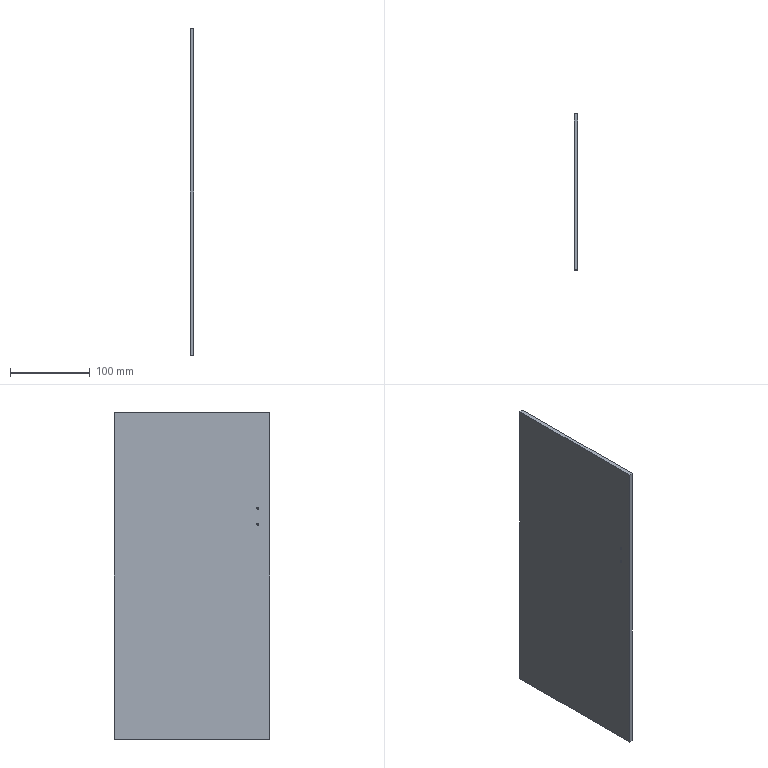Part | STEP file | 09-08 Outer side plate 1 | 1 solid | 10 faces | box 5 x 195 x 410 mm | volume 399701 mm3 | plane 6 | cylinder 4 | commonest cylinder face diameters 2.5 x4
STEP:
#1=CARTESIAN_POINT('',(0.,0.,0.));
#2=DIRECTION('',(0.,0.,1.));
#3=DIRECTION('',(1.,0.,0.));
#4=AXIS2_PLACEMENT_3D('',#1,#2,#3);
#5=CARTESIAN_POINT('',(0.,15.,-121.25));
#6=VERTEX_POINT('',#5);
#7=CARTESIAN_POINT('',(5.,15.,-121.25));
#8=VERTEX_POINT('',#7);
#9=CARTESIAN_POINT('',(0.,15.,-121.25));
#10=DIRECTION('',(1.,0.,0.));
#11=VECTOR('',#10,1.);
#12=LINE('',#9,#11);
#13=CARTESIAN_POINT('',(0.,15.,-120.));
#14=DIRECTION('',(1.,0.,0.));
#15=DIRECTION('',(0.,0.,-1.));
#16=AXIS2_PLACEMENT_3D('',#13,#14,#15);
#17=CYLINDRICAL_SURFACE('',#16,1.25);
#18=CARTESIAN_POINT('',(6.283,0.));
#19=DIRECTION('',(0.,1.));
#20=VECTOR('',#19,1.);
#21=LINE('',#18,#20);
#22=(GEOMETRIC_REPRESENTATION_CONTEXT(2)PARAMETRIC_REPRESENTATION_CONTEXT()REPRESENTATION_CONTEXT('',''));
#23=DEFINITIONAL_REPRESENTATION('',(#21),#22);
#24=PCURVE('',#17,#23);
#25=CARTESIAN_POINT('',(0.,15.,-120.));
#26=DIRECTION('',(1.,0.,0.));
#27=DIRECTION('',(0.,0.,-1.));
#28=AXIS2_PLACEMENT_3D('',#25,#26,#27);
#29=CYLINDRICAL_SURFACE('',#28,1.25);
#30=CARTESIAN_POINT('',(0.,0.));
#31=DIRECTION('',(0.,1.));
#32=VECTOR('',#31,1.);
#33=LINE('',#30,#32);
#34=(GEOMETRIC_REPRESENTATION_CONTEXT(2)PARAMETRIC_REPRESENTATION_CONTEXT()REPRESENTATION_CONTEXT('',''));
#35=DEFINITIONAL_REPRESENTATION('',(#33),#34);
#36=PCURVE('',#29,#35);
#37=SURFACE_CURVE('',#12,(#24,#36),.PCURVE_S1.);
#38=EDGE_CURVE('',#6,#8,#37,.T.);
#39=ORIENTED_EDGE('',*,*,#38,.T.);
#40=CARTESIAN_POINT('',(5.,15.,-118.75));
#41=VERTEX_POINT('',#40);
#42=CARTESIAN_POINT('',(5.,15.,-120.));
#43=DIRECTION('',(1.,0.,0.));
#44=DIRECTION('',(0.,0.,-1.));
#45=AXIS2_PLACEMENT_3D('',#42,#43,#44);
#46=CIRCLE('',#45,1.25);
#47=CARTESIAN_POINT('',(0.,5.));
#48=DIRECTION('',(1.,0.));
#49=VECTOR('',#48,1.);
#50=LINE('',#47,#49);
#51=(GEOMETRIC_REPRESENTATION_CONTEXT(2)PARAMETRIC_REPRESENTATION_CONTEXT()REPRESENTATION_CONTEXT('',''));
#52=DEFINITIONAL_REPRESENTATION('',(#50),#51);
#53=PCURVE('',#17,#52);
#54=CARTESIAN_POINT('',(5.,0.,-410.));
#55=DIRECTION('',(-1.,0.,0.));
#56=DIRECTION('',(0.,0.,1.));
#57=AXIS2_PLACEMENT_3D('',#54,#55,#56);
#58=PLANE('',#57);
#59=CARTESIAN_POINT('',(288.75,15.));
#60=CARTESIAN_POINT('',(288.75,17.165));
#61=CARTESIAN_POINT('',(290.625,16.083));
#62=CARTESIAN_POINT('',(292.5,15.));
#63=CARTESIAN_POINT('',(290.625,13.917));
#64=CARTESIAN_POINT('',(288.75,12.835));
#65=CARTESIAN_POINT('',(288.75,15.));
#66=(BOUNDED_CURVE()B_SPLINE_CURVE(2,(#59,#60,#61,#62,#63,#64,#65),.UNSPECIFIED.,.T.,.F.)B_SPLINE_CURVE_WITH_KNOTS((1,2,2,2,2,1),(-2.094,0.,2.094,4.189,6.283,8.378),.UNSPECIFIED.)CURVE()GEOMETRIC_REPRESENTATION_ITEM()RATIONAL_B_SPLINE_CURVE((1.,0.5,1.,0.5,1.,0.5,1.))REPRESENTATION_ITEM(''));
#67=(GEOMETRIC_REPRESENTATION_CONTEXT(2)PARAMETRIC_REPRESENTATION_CONTEXT()REPRESENTATION_CONTEXT('',''));
#68=DEFINITIONAL_REPRESENTATION('',(#66),#67);
#69=PCURVE('',#58,#68);
#70=SURFACE_CURVE('',#46,(#53,#69),.PCURVE_S1.);
#71=EDGE_CURVE('',#41,#8,#70,.T.);
#72=ORIENTED_EDGE('',*,*,#71,.F.);
#73=CARTESIAN_POINT('',(0.,15.,-118.75));
#74=VERTEX_POINT('',#73);
#75=CARTESIAN_POINT('',(0.,15.,-118.75));
#76=DIRECTION('',(1.,0.,0.));
#77=VECTOR('',#76,1.);
#78=LINE('',#75,#77);
#79=CARTESIAN_POINT('',(3.142,0.));
#80=DIRECTION('',(0.,1.));
#81=VECTOR('',#80,1.);
#82=LINE('',#79,#81);
#83=(GEOMETRIC_REPRESENTATION_CONTEXT(2)PARAMETRIC_REPRESENTATION_CONTEXT()REPRESENTATION_CONTEXT('',''));
#84=DEFINITIONAL_REPRESENTATION('',(#82),#83);
#85=PCURVE('',#17,#84);
#86=CARTESIAN_POINT('',(3.142,0.));
#87=DIRECTION('',(0.,1.));
#88=VECTOR('',#87,1.);
#89=LINE('',#86,#88);
#90=(GEOMETRIC_REPRESENTATION_CONTEXT(2)PARAMETRIC_REPRESENTATION_CONTEXT()REPRESENTATION_CONTEXT('',''));
#91=DEFINITIONAL_REPRESENTATION('',(#89),#90);
#92=PCURVE('',#29,#91);
#93=SURFACE_CURVE('',#78,(#85,#92),.PCURVE_S1.);
#94=EDGE_CURVE('',#74,#41,#93,.T.);
#95=ORIENTED_EDGE('',*,*,#94,.F.);
#96=CARTESIAN_POINT('',(0.,15.,-120.));
#97=DIRECTION('',(-1.,0.,0.));
#98=DIRECTION('',(0.,0.,-1.));
#99=AXIS2_PLACEMENT_3D('',#96,#97,#98);
#100=CIRCLE('',#99,1.25);
#101=CARTESIAN_POINT('',(6.283,0.));
#102=DIRECTION('',(-1.,0.));
#103=VECTOR('',#102,1.);
#104=LINE('',#101,#103);
#105=(GEOMETRIC_REPRESENTATION_CONTEXT(2)PARAMETRIC_REPRESENTATION_CONTEXT()REPRESENTATION_CONTEXT('',''));
#106=DEFINITIONAL_REPRESENTATION('',(#104),#105);
#107=PCURVE('',#17,#106);
#108=CARTESIAN_POINT('',(0.,0.,-410.));
#109=DIRECTION('',(-1.,0.,0.));
#110=DIRECTION('',(0.,0.,1.));
#111=AXIS2_PLACEMENT_3D('',#108,#109,#110);
#112=PLANE('',#111);
#113=CARTESIAN_POINT('',(290.,15.));
#114=DIRECTION('',(-1.,0.));
#115=AXIS2_PLACEMENT_2D('',#113,#114);
#116=CIRCLE('',#115,1.25);
#117=(GEOMETRIC_REPRESENTATION_CONTEXT(2)PARAMETRIC_REPRESENTATION_CONTEXT()REPRESENTATION_CONTEXT('',''));
#118=DEFINITIONAL_REPRESENTATION('',(#116),#117);
#119=PCURVE('',#112,#118);
#120=SURFACE_CURVE('',#100,(#107,#119),.PCURVE_S1.);
#121=EDGE_CURVE('',#6,#74,#120,.T.);
#122=ORIENTED_EDGE('',*,*,#121,.F.);
#123=EDGE_LOOP('',(#39,#72,#95,#122));
#124=FACE_BOUND('',#123,.F.);
#125=ADVANCED_FACE('',(#124),#17,.F.);
#126=CARTESIAN_POINT('',(0.,15.,-141.25));
#127=VERTEX_POINT('',#126);
#128=CARTESIAN_POINT('',(5.,15.,-141.25));
#129=VERTEX_POINT('',#128);
#130=CARTESIAN_POINT('',(0.,15.,-141.25));
#131=DIRECTION('',(1.,0.,0.));
#132=VECTOR('',#131,1.);
#133=LINE('',#130,#132);
#134=CARTESIAN_POINT('',(0.,15.,-140.));
#135=DIRECTION('',(1.,0.,0.));
#136=DIRECTION('',(0.,0.,-1.));
#137=AXIS2_PLACEMENT_3D('',#134,#135,#136);
#138=CYLINDRICAL_SURFACE('',#137,1.25);
#139=CARTESIAN_POINT('',(6.283,0.));
#140=DIRECTION('',(0.,1.));
#141=VECTOR('',#140,1.);
#142=LINE('',#139,#141);
#143=(GEOMETRIC_REPRESENTATION_CONTEXT(2)PARAMETRIC_REPRESENTATION_CONTEXT()REPRESENTATION_CONTEXT('',''));
#144=DEFINITIONAL_REPRESENTATION('',(#142),#143);
#145=PCURVE('',#138,#144);
#146=CARTESIAN_POINT('',(0.,15.,-140.));
#147=DIRECTION('',(1.,0.,0.));
#148=DIRECTION('',(0.,0.,-1.));
#149=AXIS2_PLACEMENT_3D('',#146,#147,#148);
#150=CYLINDRICAL_SURFACE('',#149,1.25);
#151=CARTESIAN_POINT('',(0.,0.));
#152=DIRECTION('',(0.,1.));
#153=VECTOR('',#152,1.);
#154=LINE('',#151,#153);
#155=(GEOMETRIC_REPRESENTATION_CONTEXT(2)PARAMETRIC_REPRESENTATION_CONTEXT()REPRESENTATION_CONTEXT('',''));
#156=DEFINITIONAL_REPRESENTATION('',(#154),#155);
#157=PCURVE('',#150,#156);
#158=SURFACE_CURVE('',#133,(#145,#157),.PCURVE_S1.);
#159=EDGE_CURVE('',#127,#129,#158,.T.);
#160=ORIENTED_EDGE('',*,*,#159,.T.);
#161=CARTESIAN_POINT('',(5.,15.,-138.75));
#162=VERTEX_POINT('',#161);
#163=CARTESIAN_POINT('',(5.,15.,-140.));
#164=DIRECTION('',(1.,0.,0.));
#165=DIRECTION('',(0.,0.,-1.));
#166=AXIS2_PLACEMENT_3D('',#163,#164,#165);
#167=CIRCLE('',#166,1.25);
#168=CARTESIAN_POINT('',(0.,5.));
#169=DIRECTION('',(1.,0.));
#170=VECTOR('',#169,1.);
#171=LINE('',#168,#170);
#172=(GEOMETRIC_REPRESENTATION_CONTEXT(2)PARAMETRIC_REPRESENTATION_CONTEXT()REPRESENTATION_CONTEXT('',''));
#173=DEFINITIONAL_REPRESENTATION('',(#171),#172);
#174=PCURVE('',#138,#173);
#175=CARTESIAN_POINT('',(268.75,15.));
#176=CARTESIAN_POINT('',(268.75,17.165));
#177=CARTESIAN_POINT('',(270.625,16.083));
#178=CARTESIAN_POINT('',(272.5,15.));
#179=CARTESIAN_POINT('',(270.625,13.917));
#180=CARTESIAN_POINT('',(268.75,12.835));
#181=CARTESIAN_POINT('',(268.75,15.));
#182=(BOUNDED_CURVE()B_SPLINE_CURVE(2,(#175,#176,#177,#178,#179,#180,#181),.UNSPECIFIED.,.T.,.F.)B_SPLINE_CURVE_WITH_KNOTS((1,2,2,2,2,1),(-2.094,0.,2.094,4.189,6.283,8.378),.UNSPECIFIED.)CURVE()GEOMETRIC_REPRESENTATION_ITEM()RATIONAL_B_SPLINE_CURVE((1.,0.5,1.,0.5,1.,0.5,1.))REPRESENTATION_ITEM(''));
#183=(GEOMETRIC_REPRESENTATION_CONTEXT(2)PARAMETRIC_REPRESENTATION_CONTEXT()REPRESENTATION_CONTEXT('',''));
#184=DEFINITIONAL_REPRESENTATION('',(#182),#183);
#185=PCURVE('',#58,#184);
#186=SURFACE_CURVE('',#167,(#174,#185),.PCURVE_S1.);
#187=EDGE_CURVE('',#162,#129,#186,.T.);
#188=ORIENTED_EDGE('',*,*,#187,.F.);
#189=CARTESIAN_POINT('',(0.,15.,-138.75));
#190=VERTEX_POINT('',#189);
#191=CARTESIAN_POINT('',(0.,15.,-138.75));
#192=DIRECTION('',(1.,0.,0.));
#193=VECTOR('',#192,1.);
#194=LINE('',#191,#193);
#195=CARTESIAN_POINT('',(3.142,0.));
#196=DIRECTION('',(0.,1.));
#197=VECTOR('',#196,1.);
#198=LINE('',#195,#197);
#199=(GEOMETRIC_REPRESENTATION_CONTEXT(2)PARAMETRIC_REPRESENTATION_CONTEXT()REPRESENTATION_CONTEXT('',''));
#200=DEFINITIONAL_REPRESENTATION('',(#198),#199);
#201=PCURVE('',#138,#200);
#202=CARTESIAN_POINT('',(3.142,0.));
#203=DIRECTION('',(0.,1.));
#204=VECTOR('',#203,1.);
#205=LINE('',#202,#204);
#206=(GEOMETRIC_REPRESENTATION_CONTEXT(2)PARAMETRIC_REPRESENTATION_CONTEXT()REPRESENTATION_CONTEXT('',''));
#207=DEFINITIONAL_REPRESENTATION('',(#205),#206);
#208=PCURVE('',#150,#207);
#209=SURFACE_CURVE('',#194,(#201,#208),.PCURVE_S1.);
#210=EDGE_CURVE('',#190,#162,#209,.T.);
#211=ORIENTED_EDGE('',*,*,#210,.F.);
#212=CARTESIAN_POINT('',(0.,15.,-140.));
#213=DIRECTION('',(1.,0.,0.));
#214=DIRECTION('',(0.,0.,-1.));
#215=AXIS2_PLACEMENT_3D('',#212,#213,#214);
#216=CIRCLE('',#215,1.25);
#217=CARTESIAN_POINT('',(0.,0.));
#218=DIRECTION('',(1.,0.));
#219=VECTOR('',#218,1.);
#220=LINE('',#217,#219);
#221=(GEOMETRIC_REPRESENTATION_CONTEXT(2)PARAMETRIC_REPRESENTATION_CONTEXT()REPRESENTATION_CONTEXT('',''));
#222=DEFINITIONAL_REPRESENTATION('',(#220),#221);
#223=PCURVE('',#138,#222);
#224=CARTESIAN_POINT('',(268.75,15.));
#225=CARTESIAN_POINT('',(268.75,17.165));
#226=CARTESIAN_POINT('',(270.625,16.083));
#227=CARTESIAN_POINT('',(272.5,15.));
#228=CARTESIAN_POINT('',(270.625,13.917));
#229=CARTESIAN_POINT('',(268.75,12.835));
#230=CARTESIAN_POINT('',(268.75,15.));
#231=(BOUNDED_CURVE()B_SPLINE_CURVE(2,(#224,#225,#226,#227,#228,#229,#230),.UNSPECIFIED.,.T.,.F.)B_SPLINE_CURVE_WITH_KNOTS((1,2,2,2,2,1),(-2.094,0.,2.094,4.189,6.283,8.378),.UNSPECIFIED.)CURVE()GEOMETRIC_REPRESENTATION_ITEM()RATIONAL_B_SPLINE_CURVE((1.,0.5,1.,0.5,1.,0.5,1.))REPRESENTATION_ITEM(''));
#232=(GEOMETRIC_REPRESENTATION_CONTEXT(2)PARAMETRIC_REPRESENTATION_CONTEXT()REPRESENTATION_CONTEXT('',''));
#233=DEFINITIONAL_REPRESENTATION('',(#231),#232);
#234=PCURVE('',#112,#233);
#235=SURFACE_CURVE('',#216,(#223,#234),.PCURVE_S1.);
#236=EDGE_CURVE('',#190,#127,#235,.T.);
#237=ORIENTED_EDGE('',*,*,#236,.T.);
#238=EDGE_LOOP('',(#160,#188,#211,#237));
#239=FACE_BOUND('',#238,.F.);
#240=ADVANCED_FACE('',(#239),#138,.F.);
#241=CARTESIAN_POINT('',(5.,15.,-120.));
#242=DIRECTION('',(1.,0.,0.));
#243=DIRECTION('',(0.,0.,-1.));
#244=AXIS2_PLACEMENT_3D('',#241,#242,#243);
#245=CIRCLE('',#244,1.25);
#246=CARTESIAN_POINT('',(0.,5.));
#247=DIRECTION('',(1.,0.));
#248=VECTOR('',#247,1.);
#249=LINE('',#246,#248);
#250=(GEOMETRIC_REPRESENTATION_CONTEXT(2)PARAMETRIC_REPRESENTATION_CONTEXT()REPRESENTATION_CONTEXT('',''));
#251=DEFINITIONAL_REPRESENTATION('',(#249),#250);
#252=PCURVE('',#29,#251);
#253=CARTESIAN_POINT('',(288.75,15.));
#254=CARTESIAN_POINT('',(288.75,17.165));
#255=CARTESIAN_POINT('',(290.625,16.083));
#256=CARTESIAN_POINT('',(292.5,15.));
#257=CARTESIAN_POINT('',(290.625,13.917));
#258=CARTESIAN_POINT('',(288.75,12.835));
#259=CARTESIAN_POINT('',(288.75,15.));
#260=(BOUNDED_CURVE()B_SPLINE_CURVE(2,(#253,#254,#255,#256,#257,#258,#259),.UNSPECIFIED.,.T.,.F.)B_SPLINE_CURVE_WITH_KNOTS((1,2,2,2,2,1),(-2.094,0.,2.094,4.189,6.283,8.378),.UNSPECIFIED.)CURVE()GEOMETRIC_REPRESENTATION_ITEM()RATIONAL_B_SPLINE_CURVE((1.,0.5,1.,0.5,1.,0.5,1.))REPRESENTATION_ITEM(''));
#261=(GEOMETRIC_REPRESENTATION_CONTEXT(2)PARAMETRIC_REPRESENTATION_CONTEXT()REPRESENTATION_CONTEXT('',''));
#262=DEFINITIONAL_REPRESENTATION('',(#260),#261);
#263=PCURVE('',#58,#262);
#264=SURFACE_CURVE('',#245,(#252,#263),.PCURVE_S1.);
#265=EDGE_CURVE('',#8,#41,#264,.T.);
#266=ORIENTED_EDGE('',*,*,#265,.F.);
#267=ORIENTED_EDGE('',*,*,#38,.F.);
#268=CARTESIAN_POINT('',(0.,15.,-120.));
#269=DIRECTION('',(-1.,0.,0.));
#270=DIRECTION('',(0.,0.,-1.));
#271=AXIS2_PLACEMENT_3D('',#268,#269,#270);
#272=CIRCLE('',#271,1.25);
#273=CARTESIAN_POINT('',(6.283,0.));
#274=DIRECTION('',(-1.,0.));
#275=VECTOR('',#274,1.);
#276=LINE('',#273,#275);
#277=(GEOMETRIC_REPRESENTATION_CONTEXT(2)PARAMETRIC_REPRESENTATION_CONTEXT()REPRESENTATION_CONTEXT('',''));
#278=DEFINITIONAL_REPRESENTATION('',(#276),#277);
#279=PCURVE('',#29,#278);
#280=CARTESIAN_POINT('',(290.,15.));
#281=DIRECTION('',(-1.,0.));
#282=AXIS2_PLACEMENT_2D('',#280,#281);
#283=CIRCLE('',#282,1.25);
#284=(GEOMETRIC_REPRESENTATION_CONTEXT(2)PARAMETRIC_REPRESENTATION_CONTEXT()REPRESENTATION_CONTEXT('',''));
#285=DEFINITIONAL_REPRESENTATION('',(#283),#284);
#286=PCURVE('',#112,#285);
#287=SURFACE_CURVE('',#272,(#279,#286),.PCURVE_S1.);
#288=EDGE_CURVE('',#74,#6,#287,.T.);
#289=ORIENTED_EDGE('',*,*,#288,.F.);
#290=ORIENTED_EDGE('',*,*,#94,.T.);
#291=EDGE_LOOP('',(#266,#267,#289,#290));
#292=FACE_BOUND('',#291,.F.);
#293=ADVANCED_FACE('',(#292),#29,.F.);
#294=CARTESIAN_POINT('',(5.,15.,-140.));
#295=DIRECTION('',(1.,0.,0.));
#296=DIRECTION('',(0.,0.,-1.));
#297=AXIS2_PLACEMENT_3D('',#294,#295,#296);
#298=CIRCLE('',#297,1.25);
#299=CARTESIAN_POINT('',(268.75,15.));
#300=CARTESIAN_POINT('',(268.75,17.165));
#301=CARTESIAN_POINT('',(270.625,16.083));
#302=CARTESIAN_POINT('',(272.5,15.));
#303=CARTESIAN_POINT('',(270.625,13.917));
#304=CARTESIAN_POINT('',(268.75,12.835));
#305=CARTESIAN_POINT('',(268.75,15.));
#306=(BOUNDED_CURVE()B_SPLINE_CURVE(2,(#299,#300,#301,#302,#303,#304,#305),.UNSPECIFIED.,.T.,.F.)B_SPLINE_CURVE_WITH_KNOTS((1,2,2,2,2,1),(-2.094,0.,2.094,4.189,6.283,8.378),.UNSPECIFIED.)CURVE()GEOMETRIC_REPRESENTATION_ITEM()RATIONAL_B_SPLINE_CURVE((1.,0.5,1.,0.5,1.,0.5,1.))REPRESENTATION_ITEM(''));
#307=(GEOMETRIC_REPRESENTATION_CONTEXT(2)PARAMETRIC_REPRESENTATION_CONTEXT()REPRESENTATION_CONTEXT('',''));
#308=DEFINITIONAL_REPRESENTATION('',(#306),#307);
#309=PCURVE('',#58,#308);
#310=CARTESIAN_POINT('',(0.,5.));
#311=DIRECTION('',(1.,0.));
#312=VECTOR('',#311,1.);
#313=LINE('',#310,#312);
#314=(GEOMETRIC_REPRESENTATION_CONTEXT(2)PARAMETRIC_REPRESENTATION_CONTEXT()REPRESENTATION_CONTEXT('',''));
#315=DEFINITIONAL_REPRESENTATION('',(#313),#314);
#316=PCURVE('',#150,#315);
#317=SURFACE_CURVE('',#298,(#309,#316),.PCURVE_S1.);
#318=EDGE_CURVE('',#129,#162,#317,.T.);
#319=ORIENTED_EDGE('',*,*,#318,.F.);
#320=ORIENTED_EDGE('',*,*,#187,.F.);
#321=EDGE_LOOP('',(#319,#320));
#322=FACE_BOUND('',#321,.T.);
#323=ORIENTED_EDGE('',*,*,#265,.F.);
#324=ORIENTED_EDGE('',*,*,#71,.F.);
#325=EDGE_LOOP('',(#323,#324));
#326=FACE_BOUND('',#325,.T.);
#327=CARTESIAN_POINT('',(5.,0.,-410.));
#328=VERTEX_POINT('',#327);
#329=CARTESIAN_POINT('',(5.,0.,0.));
#330=VERTEX_POINT('',#329);
#331=CARTESIAN_POINT('',(5.,0.,-205.));
#332=DIRECTION('',(0.,0.,1.));
#333=VECTOR('',#332,1.);
#334=LINE('',#331,#333);
#335=CARTESIAN_POINT('',(205.,0.));
#336=DIRECTION('',(1.,0.));
#337=VECTOR('',#336,1.);
#338=LINE('',#335,#337);
#339=(GEOMETRIC_REPRESENTATION_CONTEXT(2)PARAMETRIC_REPRESENTATION_CONTEXT()REPRESENTATION_CONTEXT('',''));
#340=DEFINITIONAL_REPRESENTATION('',(#338),#339);
#341=PCURVE('',#58,#340);
#342=CARTESIAN_POINT('',(0.,0.,-410.));
#343=DIRECTION('',(0.,1.,0.));
#344=DIRECTION('',(0.,0.,1.));
#345=AXIS2_PLACEMENT_3D('',#342,#343,#344);
#346=PLANE('',#345);
#347=CARTESIAN_POINT('',(205.,5.));
#348=DIRECTION('',(1.,0.));
#349=VECTOR('',#348,1.);
#350=LINE('',#347,#349);
#351=(GEOMETRIC_REPRESENTATION_CONTEXT(2)PARAMETRIC_REPRESENTATION_CONTEXT()REPRESENTATION_CONTEXT('',''));
#352=DEFINITIONAL_REPRESENTATION('',(#350),#351);
#353=PCURVE('',#346,#352);
#354=SURFACE_CURVE('',#334,(#341,#353),.PCURVE_S1.);
#355=EDGE_CURVE('',#328,#330,#354,.T.);
#356=ORIENTED_EDGE('',*,*,#355,.F.);
#357=CARTESIAN_POINT('',(5.,195.,-410.));
#358=VERTEX_POINT('',#357);
#359=CARTESIAN_POINT('',(5.,97.5,-410.));
#360=DIRECTION('',(0.,-1.,0.));
#361=VECTOR('',#360,1.);
#362=LINE('',#359,#361);
#363=CARTESIAN_POINT('',(0.,97.5));
#364=DIRECTION('',(0.,-1.));
#365=VECTOR('',#364,1.);
#366=LINE('',#363,#365);
#367=(GEOMETRIC_REPRESENTATION_CONTEXT(2)PARAMETRIC_REPRESENTATION_CONTEXT()REPRESENTATION_CONTEXT('',''));
#368=DEFINITIONAL_REPRESENTATION('',(#366),#367);
#369=PCURVE('',#58,#368);
#370=CARTESIAN_POINT('',(0.,0.,-410.));
#371=DIRECTION('',(0.,0.,1.));
#372=DIRECTION('',(1.,0.,0.));
#373=AXIS2_PLACEMENT_3D('',#370,#371,#372);
#374=PLANE('',#373);
#375=CARTESIAN_POINT('',(5.,97.5));
#376=DIRECTION('',(0.,-1.));
#377=VECTOR('',#376,1.);
#378=LINE('',#375,#377);
#379=(GEOMETRIC_REPRESENTATION_CONTEXT(2)PARAMETRIC_REPRESENTATION_CONTEXT()REPRESENTATION_CONTEXT('',''));
#380=DEFINITIONAL_REPRESENTATION('',(#378),#379);
#381=PCURVE('',#374,#380);
#382=SURFACE_CURVE('',#362,(#369,#381),.PCURVE_S1.);
#383=EDGE_CURVE('',#358,#328,#382,.T.);
#384=ORIENTED_EDGE('',*,*,#383,.F.);
#385=CARTESIAN_POINT('',(5.,195.,0.));
#386=VERTEX_POINT('',#385);
#387=CARTESIAN_POINT('',(5.,195.,-205.));
#388=DIRECTION('',(0.,0.,-1.));
#389=VECTOR('',#388,1.);
#390=LINE('',#387,#389);
#391=CARTESIAN_POINT('',(205.,195.));
#392=DIRECTION('',(-1.,0.));
#393=VECTOR('',#392,1.);
#394=LINE('',#391,#393);
#395=(GEOMETRIC_REPRESENTATION_CONTEXT(2)PARAMETRIC_REPRESENTATION_CONTEXT()REPRESENTATION_CONTEXT('',''));
#396=DEFINITIONAL_REPRESENTATION('',(#394),#395);
#397=PCURVE('',#58,#396);
#398=CARTESIAN_POINT('',(0.,195.,0.));
#399=DIRECTION('',(0.,-1.,0.));
#400=DIRECTION('',(0.,0.,-1.));
#401=AXIS2_PLACEMENT_3D('',#398,#399,#400);
#402=PLANE('',#401);
#403=CARTESIAN_POINT('',(205.,5.));
#404=DIRECTION('',(1.,0.));
#405=VECTOR('',#404,1.);
#406=LINE('',#403,#405);
#407=(GEOMETRIC_REPRESENTATION_CONTEXT(2)PARAMETRIC_REPRESENTATION_CONTEXT()REPRESENTATION_CONTEXT('',''));
#408=DEFINITIONAL_REPRESENTATION('',(#406),#407);
#409=PCURVE('',#402,#408);
#410=SURFACE_CURVE('',#390,(#397,#409),.PCURVE_S1.);
#411=EDGE_CURVE('',#386,#358,#410,.T.);
#412=ORIENTED_EDGE('',*,*,#411,.F.);
#413=CARTESIAN_POINT('',(5.,97.5,0.));
#414=DIRECTION('',(0.,1.,0.));
#415=VECTOR('',#414,1.);
#416=LINE('',#413,#415);
#417=CARTESIAN_POINT('',(410.,97.5));
#418=DIRECTION('',(0.,1.));
#419=VECTOR('',#418,1.);
#420=LINE('',#417,#419);
#421=(GEOMETRIC_REPRESENTATION_CONTEXT(2)PARAMETRIC_REPRESENTATION_CONTEXT()REPRESENTATION_CONTEXT('',''));
#422=DEFINITIONAL_REPRESENTATION('',(#420),#421);
#423=PCURVE('',#58,#422);
#424=CARTESIAN_POINT('',(5.,0.,0.));
#425=DIRECTION('',(0.,0.,-1.));
#426=DIRECTION('',(-1.,0.,0.));
#427=AXIS2_PLACEMENT_3D('',#424,#425,#426);
#428=PLANE('',#427);
#429=CARTESIAN_POINT('',(0.,97.5));
#430=DIRECTION('',(0.,1.));
#431=VECTOR('',#430,1.);
#432=LINE('',#429,#431);
#433=(GEOMETRIC_REPRESENTATION_CONTEXT(2)PARAMETRIC_REPRESENTATION_CONTEXT()REPRESENTATION_CONTEXT('',''));
#434=DEFINITIONAL_REPRESENTATION('',(#432),#433);
#435=PCURVE('',#428,#434);
#436=SURFACE_CURVE('',#416,(#423,#435),.PCURVE_S1.);
#437=EDGE_CURVE('',#330,#386,#436,.T.);
#438=ORIENTED_EDGE('',*,*,#437,.F.);
#439=EDGE_LOOP('',(#356,#384,#412,#438));
#440=FACE_BOUND('',#439,.T.);
#441=ADVANCED_FACE('',(#322,#326,#440),#58,.F.);
#442=CARTESIAN_POINT('',(0.,15.,-140.));
#443=DIRECTION('',(1.,0.,0.));
#444=DIRECTION('',(0.,0.,-1.));
#445=AXIS2_PLACEMENT_3D('',#442,#443,#444);
#446=CIRCLE('',#445,1.25);
#447=CARTESIAN_POINT('',(268.75,15.));
#448=CARTESIAN_POINT('',(268.75,17.165));
#449=CARTESIAN_POINT('',(270.625,16.083));
#450=CARTESIAN_POINT('',(272.5,15.));
#451=CARTESIAN_POINT('',(270.625,13.917));
#452=CARTESIAN_POINT('',(268.75,12.835));
#453=CARTESIAN_POINT('',(268.75,15.));
#454=(BOUNDED_CURVE()B_SPLINE_CURVE(2,(#447,#448,#449,#450,#451,#452,#453),.UNSPECIFIED.,.T.,.F.)B_SPLINE_CURVE_WITH_KNOTS((1,2,2,2,2,1),(-2.094,0.,2.094,4.189,6.283,8.378),.UNSPECIFIED.)CURVE()GEOMETRIC_REPRESENTATION_ITEM()RATIONAL_B_SPLINE_CURVE((1.,0.5,1.,0.5,1.,0.5,1.))REPRESENTATION_ITEM(''));
#455=(GEOMETRIC_REPRESENTATION_CONTEXT(2)PARAMETRIC_REPRESENTATION_CONTEXT()REPRESENTATION_CONTEXT('',''));
#456=DEFINITIONAL_REPRESENTATION('',(#454),#455);
#457=PCURVE('',#112,#456);
#458=CARTESIAN_POINT('',(0.,0.));
#459=DIRECTION('',(1.,0.));
#460=VECTOR('',#459,1.);
#461=LINE('',#458,#460);
#462=(GEOMETRIC_REPRESENTATION_CONTEXT(2)PARAMETRIC_REPRESENTATION_CONTEXT()REPRESENTATION_CONTEXT('',''));
#463=DEFINITIONAL_REPRESENTATION('',(#461),#462);
#464=PCURVE('',#150,#463);
#465=SURFACE_CURVE('',#446,(#457,#464),.PCURVE_S1.);
#466=EDGE_CURVE('',#127,#190,#465,.T.);
#467=ORIENTED_EDGE('',*,*,#466,.T.);
#468=ORIENTED_EDGE('',*,*,#236,.T.);
#469=EDGE_LOOP('',(#467,#468));
#470=FACE_BOUND('',#469,.T.);
#471=ORIENTED_EDGE('',*,*,#121,.F.);
#472=ORIENTED_EDGE('',*,*,#288,.F.);
#473=EDGE_LOOP('',(#471,#472));
#474=FACE_BOUND('',#473,.T.);
#475=CARTESIAN_POINT('',(0.,195.,-410.));
#476=VERTEX_POINT('',#475);
#477=CARTESIAN_POINT('',(0.,0.,-410.));
#478=VERTEX_POINT('',#477);
#479=CARTESIAN_POINT('',(0.,97.5,-410.));
#480=DIRECTION('',(0.,-1.,0.));
#481=VECTOR('',#480,1.);
#482=LINE('',#479,#481);
#483=CARTESIAN_POINT('',(0.,97.5));
#484=DIRECTION('',(0.,-1.));
#485=VECTOR('',#484,1.);
#486=LINE('',#483,#485);
#487=(GEOMETRIC_REPRESENTATION_CONTEXT(2)PARAMETRIC_REPRESENTATION_CONTEXT()REPRESENTATION_CONTEXT('',''));
#488=DEFINITIONAL_REPRESENTATION('',(#486),#487);
#489=PCURVE('',#112,#488);
#490=CARTESIAN_POINT('',(0.,97.5));
#491=DIRECTION('',(0.,-1.));
#492=VECTOR('',#491,1.);
#493=LINE('',#490,#492);
#494=(GEOMETRIC_REPRESENTATION_CONTEXT(2)PARAMETRIC_REPRESENTATION_CONTEXT()REPRESENTATION_CONTEXT('',''));
#495=DEFINITIONAL_REPRESENTATION('',(#493),#494);
#496=PCURVE('',#374,#495);
#497=SURFACE_CURVE('',#482,(#489,#496),.PCURVE_S1.);
#498=EDGE_CURVE('',#476,#478,#497,.T.);
#499=ORIENTED_EDGE('',*,*,#498,.T.);
#500=CARTESIAN_POINT('',(0.,0.,0.));
#501=VERTEX_POINT('',#500);
#502=CARTESIAN_POINT('',(0.,0.,-205.));
#503=DIRECTION('',(0.,0.,1.));
#504=VECTOR('',#503,1.);
#505=LINE('',#502,#504);
#506=CARTESIAN_POINT('',(205.,0.));
#507=DIRECTION('',(1.,0.));
#508=VECTOR('',#507,1.);
#509=LINE('',#506,#508);
#510=(GEOMETRIC_REPRESENTATION_CONTEXT(2)PARAMETRIC_REPRESENTATION_CONTEXT()REPRESENTATION_CONTEXT('',''));
#511=DEFINITIONAL_REPRESENTATION('',(#509),#510);
#512=PCURVE('',#112,#511);
#513=CARTESIAN_POINT('',(205.,0.));
#514=DIRECTION('',(1.,0.));
#515=VECTOR('',#514,1.);
#516=LINE('',#513,#515);
#517=(GEOMETRIC_REPRESENTATION_CONTEXT(2)PARAMETRIC_REPRESENTATION_CONTEXT()REPRESENTATION_CONTEXT('',''));
#518=DEFINITIONAL_REPRESENTATION('',(#516),#517);
#519=PCURVE('',#346,#518);
#520=SURFACE_CURVE('',#505,(#512,#519),.PCURVE_S1.);
#521=EDGE_CURVE('',#478,#501,#520,.T.);
#522=ORIENTED_EDGE('',*,*,#521,.T.);
#523=CARTESIAN_POINT('',(0.,195.,0.));
#524=VERTEX_POINT('',#523);
#525=CARTESIAN_POINT('',(0.,97.5,0.));
#526=DIRECTION('',(0.,1.,0.));
#527=VECTOR('',#526,1.);
#528=LINE('',#525,#527);
#529=CARTESIAN_POINT('',(410.,97.5));
#530=DIRECTION('',(0.,1.));
#531=VECTOR('',#530,1.);
#532=LINE('',#529,#531);
#533=(GEOMETRIC_REPRESENTATION_CONTEXT(2)PARAMETRIC_REPRESENTATION_CONTEXT()REPRESENTATION_CONTEXT('',''));
#534=DEFINITIONAL_REPRESENTATION('',(#532),#533);
#535=PCURVE('',#112,#534);
#536=CARTESIAN_POINT('',(5.,97.5));
#537=DIRECTION('',(0.,1.));
#538=VECTOR('',#537,1.);
#539=LINE('',#536,#538);
#540=(GEOMETRIC_REPRESENTATION_CONTEXT(2)PARAMETRIC_REPRESENTATION_CONTEXT()REPRESENTATION_CONTEXT('',''));
#541=DEFINITIONAL_REPRESENTATION('',(#539),#540);
#542=PCURVE('',#428,#541);
#543=SURFACE_CURVE('',#528,(#535,#542),.PCURVE_S1.);
#544=EDGE_CURVE('',#501,#524,#543,.T.);
#545=ORIENTED_EDGE('',*,*,#544,.T.);
#546=CARTESIAN_POINT('',(0.,195.,-205.));
#547=DIRECTION('',(0.,0.,-1.));
#548=VECTOR('',#547,1.);
#549=LINE('',#546,#548);
#550=CARTESIAN_POINT('',(205.,195.));
#551=DIRECTION('',(-1.,0.));
#552=VECTOR('',#551,1.);
#553=LINE('',#550,#552);
#554=(GEOMETRIC_REPRESENTATION_CONTEXT(2)PARAMETRIC_REPRESENTATION_CONTEXT()REPRESENTATION_CONTEXT('',''));
#555=DEFINITIONAL_REPRESENTATION('',(#553),#554);
#556=PCURVE('',#112,#555);
#557=CARTESIAN_POINT('',(205.,0.));
#558=DIRECTION('',(1.,0.));
#559=VECTOR('',#558,1.);
#560=LINE('',#557,#559);
#561=(GEOMETRIC_REPRESENTATION_CONTEXT(2)PARAMETRIC_REPRESENTATION_CONTEXT()REPRESENTATION_CONTEXT('',''));
#562=DEFINITIONAL_REPRESENTATION('',(#560),#561);
#563=PCURVE('',#402,#562);
#564=SURFACE_CURVE('',#549,(#556,#563),.PCURVE_S1.);
#565=EDGE_CURVE('',#524,#476,#564,.T.);
#566=ORIENTED_EDGE('',*,*,#565,.T.);
#567=EDGE_LOOP('',(#499,#522,#545,#566));
#568=FACE_BOUND('',#567,.T.);
#569=ADVANCED_FACE('',(#470,#474,#568),#112,.T.);
#570=ORIENTED_EDGE('',*,*,#318,.F.);
#571=ORIENTED_EDGE('',*,*,#159,.F.);
#572=ORIENTED_EDGE('',*,*,#466,.T.);
#573=ORIENTED_EDGE('',*,*,#210,.T.);
#574=EDGE_LOOP('',(#570,#571,#572,#573));
#575=FACE_BOUND('',#574,.F.);
#576=ADVANCED_FACE('',(#575),#150,.F.);
#577=CARTESIAN_POINT('',(2.5,0.,0.));
#578=DIRECTION('',(-1.,0.,0.));
#579=VECTOR('',#578,1.);
#580=LINE('',#577,#579);
#581=CARTESIAN_POINT('',(2.5,0.));
#582=DIRECTION('',(1.,0.));
#583=VECTOR('',#582,1.);
#584=LINE('',#581,#583);
#585=(GEOMETRIC_REPRESENTATION_CONTEXT(2)PARAMETRIC_REPRESENTATION_CONTEXT()REPRESENTATION_CONTEXT('',''));
#586=DEFINITIONAL_REPRESENTATION('',(#584),#585);
#587=PCURVE('',#428,#586);
#588=CARTESIAN_POINT('',(410.,2.5));
#589=DIRECTION('',(0.,-1.));
#590=VECTOR('',#589,1.);
#591=LINE('',#588,#590);
#592=(GEOMETRIC_REPRESENTATION_CONTEXT(2)PARAMETRIC_REPRESENTATION_CONTEXT()REPRESENTATION_CONTEXT('',''));
#593=DEFINITIONAL_REPRESENTATION('',(#591),#592);
#594=PCURVE('',#346,#593);
#595=SURFACE_CURVE('',#580,(#587,#594),.PCURVE_S1.);
#596=EDGE_CURVE('',#330,#501,#595,.T.);
#597=ORIENTED_EDGE('',*,*,#596,.F.);
#598=ORIENTED_EDGE('',*,*,#437,.T.);
#599=CARTESIAN_POINT('',(2.5,195.,0.));
#600=DIRECTION('',(1.,0.,0.));
#601=VECTOR('',#600,1.);
#602=LINE('',#599,#601);
#603=CARTESIAN_POINT('',(2.5,195.));
#604=DIRECTION('',(-1.,0.));
#605=VECTOR('',#604,1.);
#606=LINE('',#603,#605);
#607=(GEOMETRIC_REPRESENTATION_CONTEXT(2)PARAMETRIC_REPRESENTATION_CONTEXT()REPRESENTATION_CONTEXT('',''));
#608=DEFINITIONAL_REPRESENTATION('',(#606),#607);
#609=PCURVE('',#428,#608);
#610=CARTESIAN_POINT('',(0.,2.5));
#611=DIRECTION('',(0.,1.));
#612=VECTOR('',#611,1.);
#613=LINE('',#610,#612);
#614=(GEOMETRIC_REPRESENTATION_CONTEXT(2)PARAMETRIC_REPRESENTATION_CONTEXT()REPRESENTATION_CONTEXT('',''));
#615=DEFINITIONAL_REPRESENTATION('',(#613),#614);
#616=PCURVE('',#402,#615);
#617=SURFACE_CURVE('',#602,(#609,#616),.PCURVE_S1.);
#618=EDGE_CURVE('',#524,#386,#617,.T.);
#619=ORIENTED_EDGE('',*,*,#618,.F.);
#620=ORIENTED_EDGE('',*,*,#544,.F.);
#621=EDGE_LOOP('',(#597,#598,#619,#620));
#622=FACE_BOUND('',#621,.T.);
#623=ADVANCED_FACE('',(#622),#428,.F.);
#624=CARTESIAN_POINT('',(2.5,0.,-410.));
#625=DIRECTION('',(-1.,0.,0.));
#626=VECTOR('',#625,1.);
#627=LINE('',#624,#626);
#628=CARTESIAN_POINT('',(0.,2.5));
#629=DIRECTION('',(0.,-1.));
#630=VECTOR('',#629,1.);
#631=LINE('',#628,#630);
#632=(GEOMETRIC_REPRESENTATION_CONTEXT(2)PARAMETRIC_REPRESENTATION_CONTEXT()REPRESENTATION_CONTEXT('',''));
#633=DEFINITIONAL_REPRESENTATION('',(#631),#632);
#634=PCURVE('',#346,#633);
#635=CARTESIAN_POINT('',(2.5,0.));
#636=DIRECTION('',(-1.,0.));
#637=VECTOR('',#636,1.);
#638=LINE('',#635,#637);
#639=(GEOMETRIC_REPRESENTATION_CONTEXT(2)PARAMETRIC_REPRESENTATION_CONTEXT()REPRESENTATION_CONTEXT('',''));
#640=DEFINITIONAL_REPRESENTATION('',(#638),#639);
#641=PCURVE('',#374,#640);
#642=SURFACE_CURVE('',#627,(#634,#641),.PCURVE_S1.);
#643=EDGE_CURVE('',#328,#478,#642,.T.);
#644=ORIENTED_EDGE('',*,*,#643,.F.);
#645=ORIENTED_EDGE('',*,*,#355,.T.);
#646=ORIENTED_EDGE('',*,*,#596,.T.);
#647=ORIENTED_EDGE('',*,*,#521,.F.);
#648=EDGE_LOOP('',(#644,#645,#646,#647));
#649=FACE_BOUND('',#648,.T.);
#650=ADVANCED_FACE('',(#649),#346,.F.);
#651=CARTESIAN_POINT('',(2.5,195.,-410.));
#652=DIRECTION('',(-1.,0.,0.));
#653=VECTOR('',#652,1.);
#654=LINE('',#651,#653);
#655=CARTESIAN_POINT('',(2.5,195.));
#656=DIRECTION('',(-1.,0.));
#657=VECTOR('',#656,1.);
#658=LINE('',#655,#657);
#659=(GEOMETRIC_REPRESENTATION_CONTEXT(2)PARAMETRIC_REPRESENTATION_CONTEXT()REPRESENTATION_CONTEXT('',''));
#660=DEFINITIONAL_REPRESENTATION('',(#658),#659);
#661=PCURVE('',#374,#660);
#662=CARTESIAN_POINT('',(410.,2.5));
#663=DIRECTION('',(0.,-1.));
#664=VECTOR('',#663,1.);
#665=LINE('',#662,#664);
#666=(GEOMETRIC_REPRESENTATION_CONTEXT(2)PARAMETRIC_REPRESENTATION_CONTEXT()REPRESENTATION_CONTEXT('',''));
#667=DEFINITIONAL_REPRESENTATION('',(#665),#666);
#668=PCURVE('',#402,#667);
#669=SURFACE_CURVE('',#654,(#661,#668),.PCURVE_S1.);
#670=EDGE_CURVE('',#358,#476,#669,.T.);
#671=ORIENTED_EDGE('',*,*,#670,.F.);
#672=ORIENTED_EDGE('',*,*,#383,.T.);
#673=ORIENTED_EDGE('',*,*,#643,.T.);
#674=ORIENTED_EDGE('',*,*,#498,.F.);
#675=EDGE_LOOP('',(#671,#672,#673,#674));
#676=FACE_BOUND('',#675,.T.);
#677=ADVANCED_FACE('',(#676),#374,.F.);
#678=ORIENTED_EDGE('',*,*,#618,.T.);
#679=ORIENTED_EDGE('',*,*,#411,.T.);
#680=ORIENTED_EDGE('',*,*,#670,.T.);
#681=ORIENTED_EDGE('',*,*,#565,.F.);
#682=EDGE_LOOP('',(#678,#679,#680,#681));
#683=FACE_BOUND('',#682,.T.);
#684=ADVANCED_FACE('',(#683),#402,.F.);
#685=CLOSED_SHELL('',(#125,#240,#293,#441,#569,#576,#623,#650,#677,#684));
#686=MANIFOLD_SOLID_BREP('',#685);
#687=(LENGTH_UNIT()NAMED_UNIT(*)SI_UNIT(.MILLI.,.METRE.));
#688=UNCERTAINTY_MEASURE_WITH_UNIT(LENGTH_MEASURE(0.0000001),#687,'','');
#689=(NAMED_UNIT(*)PLANE_ANGLE_UNIT()SI_UNIT($,.RADIAN.));
#690=(NAMED_UNIT(*)SI_UNIT($,.STERADIAN.)SOLID_ANGLE_UNIT());
#691=(GEOMETRIC_REPRESENTATION_CONTEXT(3)GLOBAL_UNCERTAINTY_ASSIGNED_CONTEXT((#688))GLOBAL_UNIT_ASSIGNED_CONTEXT((#687,#689,#690))REPRESENTATION_CONTEXT('',''));
#692=ADVANCED_BREP_SHAPE_REPRESENTATION('',(#4,#686),#691);